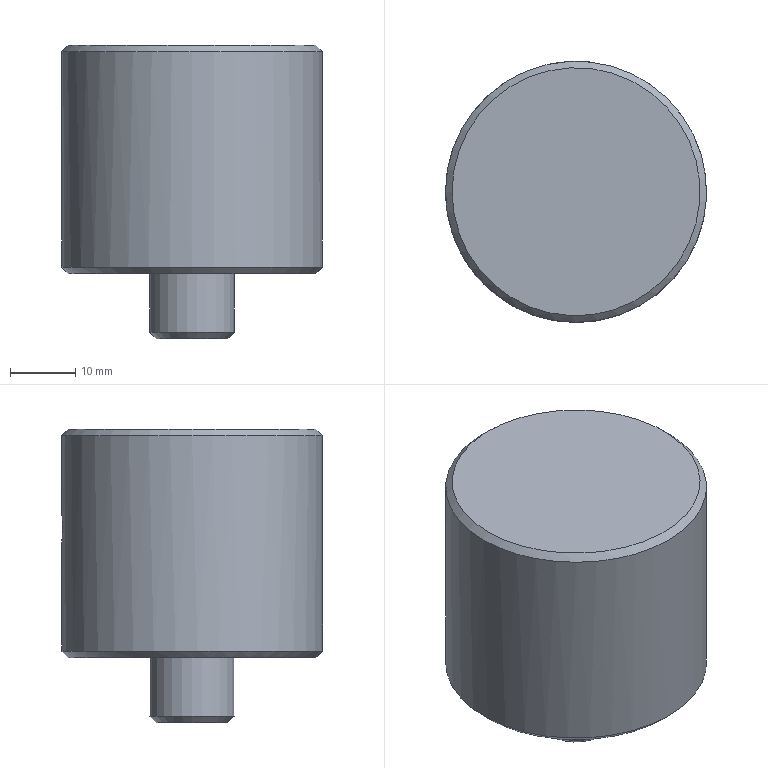Part | STEP file | gslz 2016.10.28-6_id186_x_t | 1 solid | 10 faces | box 40 x 40 x 45 mm | volume 44861 mm3 | cone 4 | cylinder 3 | plane 3 | commonest cylinder face diameters 5 x1 13 x1 40 x1
STEP:
#1=CARTESIAN_POINT('',(-310.,130.,30.992));
#2=VERTEX_POINT('',#1);
#3=CARTESIAN_POINT('',(-310.,150.,30.992));
#4=DIRECTION('',(0.,0.,-1.));
#5=DIRECTION('',(0.,-1.,0.));
#6=AXIS2_PLACEMENT_3D('',#3,#4,#5);
#7=CIRCLE('',#6,20.);
#8=EDGE_CURVE('',#2,#2,#7,.T.);
#9=ORIENTED_EDGE('',*,*,#8,.F.);
#10=EDGE_LOOP('',(#9));
#11=FACE_BOUND('',#10,.T.);
#12=CARTESIAN_POINT('',(-310.,130.,63.992));
#13=VERTEX_POINT('',#12);
#14=CARTESIAN_POINT('',(-310.,150.,63.992));
#15=DIRECTION('',(0.,0.,1.));
#16=DIRECTION('',(0.,-1.,0.));
#17=AXIS2_PLACEMENT_3D('',#14,#15,#16);
#18=CIRCLE('',#17,20.);
#19=EDGE_CURVE('',#13,#13,#18,.T.);
#20=ORIENTED_EDGE('',*,*,#19,.F.);
#21=EDGE_LOOP('',(#20));
#22=FACE_BOUND('',#21,.T.);
#23=CARTESIAN_POINT('',(-308.582,169.95,52.053));
#24=VERTEX_POINT('',#23);
#25=CARTESIAN_POINT('',(-308.582,169.95,52.053));
#26=CARTESIAN_POINT('',(-308.351,169.933,51.894));
#27=CARTESIAN_POINT('',(-308.145,169.914,51.693));
#28=CARTESIAN_POINT('',(-307.979,169.898,51.467));
#29=CARTESIAN_POINT('',(-307.814,169.881,51.241));
#30=CARTESIAN_POINT('',(-307.686,169.866,50.983));
#31=CARTESIAN_POINT('',(-307.605,169.856,50.714));
#32=CARTESIAN_POINT('',(-307.524,169.846,50.446));
#33=CARTESIAN_POINT('',(-307.488,169.842,50.161));
#34=CARTESIAN_POINT('',(-307.501,169.843,49.881));
#35=CARTESIAN_POINT('',(-307.513,169.845,49.604));
#36=CARTESIAN_POINT('',(-307.573,169.853,49.324));
#37=CARTESIAN_POINT('',(-307.676,169.865,49.066));
#38=CARTESIAN_POINT('',(-307.779,169.877,48.808));
#39=CARTESIAN_POINT('',(-307.928,169.893,48.564));
#40=CARTESIAN_POINT('',(-308.11,169.91,48.355));
#41=CARTESIAN_POINT('',(-308.293,169.928,48.143));
#42=CARTESIAN_POINT('',(-308.515,169.946,47.961));
#43=CARTESIAN_POINT('',(-308.758,169.961,47.822));
#44=CARTESIAN_POINT('',(-309.001,169.977,47.683));
#45=CARTESIAN_POINT('',(-309.272,169.989,47.584));
#46=CARTESIAN_POINT('',(-309.548,169.995,47.533));
#47=CARTESIAN_POINT('',(-309.823,170.001,47.483));
#48=CARTESIAN_POINT('',(-310.11,170.002,47.479));
#49=CARTESIAN_POINT('',(-310.385,169.996,47.523));
#50=CARTESIAN_POINT('',(-310.66,169.991,47.566));
#51=CARTESIAN_POINT('',(-310.93,169.98,47.656));
#52=CARTESIAN_POINT('',(-311.175,169.965,47.787));
#53=CARTESIAN_POINT('',(-311.421,169.951,47.918));
#54=CARTESIAN_POINT('',(-311.647,169.933,48.093));
#55=CARTESIAN_POINT('',(-311.836,169.916,48.297));
#56=CARTESIAN_POINT('',(-312.026,169.898,48.503));
#57=CARTESIAN_POINT('',(-312.183,169.881,48.744));
#58=CARTESIAN_POINT('',(-312.294,169.868,49.002));
#59=CARTESIAN_POINT('',(-312.405,169.855,49.259));
#60=CARTESIAN_POINT('',(-312.473,169.847,49.539));
#61=CARTESIAN_POINT('',(-312.492,169.844,49.819));
#62=CARTESIAN_POINT('',(-312.512,169.842,50.097));
#63=CARTESIAN_POINT('',(-312.484,169.845,50.382));
#64=CARTESIAN_POINT('',(-312.41,169.854,50.65));
#65=CARTESIAN_POINT('',(-312.337,169.863,50.918));
#66=CARTESIAN_POINT('',(-312.217,169.877,51.177));
#67=CARTESIAN_POINT('',(-312.061,169.894,51.406));
#68=CARTESIAN_POINT('',(-311.903,169.91,51.636));
#69=CARTESIAN_POINT('',(-311.704,169.929,51.842));
#70=CARTESIAN_POINT('',(-311.479,169.945,52.007));
#71=CARTESIAN_POINT('',(-311.253,169.962,52.173));
#72=CARTESIAN_POINT('',(-310.995,169.977,52.302));
#73=CARTESIAN_POINT('',(-310.727,169.987,52.384));
#74=CARTESIAN_POINT('',(-310.459,169.997,52.466));
#75=CARTESIAN_POINT('',(-310.174,170.001,52.502));
#76=CARTESIAN_POINT('',(-309.894,170.,52.49));
#77=CARTESIAN_POINT('',(-309.616,169.998,52.479));
#78=CARTESIAN_POINT('',(-309.337,169.991,52.419));
#79=CARTESIAN_POINT('',(-309.079,169.979,52.317));
#80=CARTESIAN_POINT('',(-308.904,169.971,52.248));
#81=CARTESIAN_POINT('',(-308.737,169.961,52.159));
#82=CARTESIAN_POINT('',(-308.582,169.95,52.053));
#83=B_SPLINE_CURVE_WITH_KNOTS('',3,(#25,#26,#27,#28,#29,#30,#31,#32,#33,#34,#35,#36,#37,#38,#39,#40,#41,#42,#43,#44,#45,#46,#47,#48,#49,#50,#51,#52,#53,#54,#55,#56,#57,#58,#59,#60,#61,#62,#63,#64,#65,#66,#67,#68,#69,#70,#71,#72,#73,#74,#75,#76,#77,#78,#79,#80,#81,#82),.UNSPECIFIED.,.T.,.F.,(1,3,3,3,3,3,3,3,3,3,3,3,3,3,3,3,3,3,3,3,3,1),(-0.03573,0.,0.05381,0.1076,0.1613,0.2146,0.2679,0.3216,0.3755,0.429,0.4822,0.5357,0.5895,0.6432,0.6966,0.7499,0.8035,0.8573,0.911,0.9643,1.,1.054),.UNSPECIFIED.);
#84=EDGE_CURVE('',#24,#24,#83,.T.);
#85=ORIENTED_EDGE('',*,*,#84,.F.);
#86=EDGE_LOOP('',(#85));
#87=FACE_BOUND('',#86,.T.);
#88=CARTESIAN_POINT('',(-310.,150.,69.992));
#89=DIRECTION('',(0.,0.,-1.));
#90=DIRECTION('',(-1.,0.,0.));
#91=AXIS2_PLACEMENT_3D('',#88,#89,#90);
#92=CYLINDRICAL_SURFACE('',#91,20.);
#93=ADVANCED_FACE('',(#11,#22,#87),#92,.T.);
#94=CARTESIAN_POINT('',(-303.5,150.,29.992));
#95=VERTEX_POINT('',#94);
#96=CARTESIAN_POINT('',(-310.,150.,29.992));
#97=DIRECTION('',(0.,0.,1.));
#98=DIRECTION('',(1.,0.,0.));
#99=AXIS2_PLACEMENT_3D('',#96,#97,#98);
#100=CIRCLE('',#99,6.5);
#101=EDGE_CURVE('',#95,#95,#100,.T.);
#102=ORIENTED_EDGE('',*,*,#101,.T.);
#103=EDGE_LOOP('',(#102));
#104=FACE_BOUND('',#103,.T.);
#105=CARTESIAN_POINT('',(-329.,150.,29.992));
#106=VERTEX_POINT('',#105);
#107=CARTESIAN_POINT('',(-310.,150.,29.992));
#108=DIRECTION('',(0.,0.,1.));
#109=DIRECTION('',(-1.,0.,0.));
#110=AXIS2_PLACEMENT_3D('',#107,#108,#109);
#111=CIRCLE('',#110,19.);
#112=EDGE_CURVE('',#106,#106,#111,.T.);
#113=ORIENTED_EDGE('',*,*,#112,.F.);
#114=EDGE_LOOP('',(#113));
#115=FACE_BOUND('',#114,.T.);
#116=CARTESIAN_POINT('',(-310.,150.,29.992));
#117=DIRECTION('',(0.,0.,1.));
#118=DIRECTION('',(0.,1.,0.));
#119=AXIS2_PLACEMENT_3D('',#116,#117,#118);
#120=PLANE('',#119);
#121=ADVANCED_FACE('',(#104,#115),#120,.F.);
#122=CARTESIAN_POINT('',(-329.,150.,64.992));
#123=VERTEX_POINT('',#122);
#124=CARTESIAN_POINT('',(-310.,150.,64.992));
#125=DIRECTION('',(0.,0.,-1.));
#126=DIRECTION('',(-1.,0.,0.));
#127=AXIS2_PLACEMENT_3D('',#124,#125,#126);
#128=CIRCLE('',#127,19.);
#129=EDGE_CURVE('',#123,#123,#128,.T.);
#130=ORIENTED_EDGE('',*,*,#129,.F.);
#131=EDGE_LOOP('',(#130));
#132=FACE_OUTER_BOUND('',#131,.T.);
#133=CARTESIAN_POINT('',(-310.,150.,64.992));
#134=DIRECTION('',(0.,0.,1.));
#135=DIRECTION('',(0.,1.,0.));
#136=AXIS2_PLACEMENT_3D('',#133,#134,#135);
#137=PLANE('',#136);
#138=ADVANCED_FACE('',(#132),#137,.T.);
#139=ORIENTED_EDGE('',*,*,#84,.T.);
#140=EDGE_LOOP('',(#139));
#141=FACE_BOUND('',#140,.T.);
#142=CARTESIAN_POINT('',(-307.499,154.9,49.992));
#143=VERTEX_POINT('',#142);
#144=CARTESIAN_POINT('',(-307.499,154.9,49.992));
#145=CARTESIAN_POINT('',(-307.499,154.9,50.272));
#146=CARTESIAN_POINT('',(-307.547,154.9,50.556));
#147=CARTESIAN_POINT('',(-307.64,154.9,50.82));
#148=CARTESIAN_POINT('',(-307.733,154.9,51.084));
#149=CARTESIAN_POINT('',(-307.872,154.9,51.336));
#150=CARTESIAN_POINT('',(-308.047,154.9,51.554));
#151=CARTESIAN_POINT('',(-308.222,154.9,51.773));
#152=CARTESIAN_POINT('',(-308.437,154.9,51.964));
#153=CARTESIAN_POINT('',(-308.674,154.9,52.112));
#154=CARTESIAN_POINT('',(-308.911,154.9,52.261));
#155=CARTESIAN_POINT('',(-309.177,154.9,52.37));
#156=CARTESIAN_POINT('',(-309.45,154.9,52.431));
#157=CARTESIAN_POINT('',(-309.723,154.9,52.493));
#158=CARTESIAN_POINT('',(-310.011,154.9,52.508));
#159=CARTESIAN_POINT('',(-310.289,154.9,52.476));
#160=CARTESIAN_POINT('',(-310.566,154.9,52.443));
#161=CARTESIAN_POINT('',(-310.843,154.9,52.362));
#162=CARTESIAN_POINT('',(-311.094,154.9,52.24));
#163=CARTESIAN_POINT('',(-311.346,154.9,52.117));
#164=CARTESIAN_POINT('',(-311.58,154.9,51.95));
#165=CARTESIAN_POINT('',(-311.776,154.9,51.751));
#166=CARTESIAN_POINT('',(-311.973,154.9,51.552));
#167=CARTESIAN_POINT('',(-312.138,154.9,51.316));
#168=CARTESIAN_POINT('',(-312.258,154.9,51.063));
#169=CARTESIAN_POINT('',(-312.378,154.9,50.81));
#170=CARTESIAN_POINT('',(-312.456,154.9,50.533));
#171=CARTESIAN_POINT('',(-312.485,154.9,50.255));
#172=CARTESIAN_POINT('',(-312.515,154.9,49.977));
#173=CARTESIAN_POINT('',(-312.496,154.9,49.69));
#174=CARTESIAN_POINT('',(-312.432,154.9,49.417));
#175=CARTESIAN_POINT('',(-312.368,154.9,49.145));
#176=CARTESIAN_POINT('',(-312.255,154.9,48.88));
#177=CARTESIAN_POINT('',(-312.105,154.9,48.645));
#178=CARTESIAN_POINT('',(-311.954,154.9,48.409));
#179=CARTESIAN_POINT('',(-311.76,154.9,48.196));
#180=CARTESIAN_POINT('',(-311.54,154.9,48.024));
#181=CARTESIAN_POINT('',(-311.319,154.9,47.851));
#182=CARTESIAN_POINT('',(-311.066,154.9,47.714));
#183=CARTESIAN_POINT('',(-310.801,154.9,47.625));
#184=CARTESIAN_POINT('',(-310.536,154.9,47.535));
#185=CARTESIAN_POINT('',(-310.252,154.9,47.49));
#186=CARTESIAN_POINT('',(-309.972,154.9,47.493));
#187=CARTESIAN_POINT('',(-309.692,154.9,47.496));
#188=CARTESIAN_POINT('',(-309.409,154.9,47.547));
#189=CARTESIAN_POINT('',(-309.146,154.9,47.642));
#190=CARTESIAN_POINT('',(-308.883,154.9,47.738));
#191=CARTESIAN_POINT('',(-308.633,154.9,47.88));
#192=CARTESIAN_POINT('',(-308.416,154.9,48.057));
#193=CARTESIAN_POINT('',(-308.2,154.9,48.234));
#194=CARTESIAN_POINT('',(-308.011,154.9,48.451));
#195=CARTESIAN_POINT('',(-307.865,154.9,48.69));
#196=CARTESIAN_POINT('',(-307.719,154.9,48.929));
#197=CARTESIAN_POINT('',(-307.613,154.9,49.196));
#198=CARTESIAN_POINT('',(-307.554,154.9,49.47));
#199=CARTESIAN_POINT('',(-307.518,154.9,49.641));
#200=CARTESIAN_POINT('',(-307.499,154.9,49.817));
#201=CARTESIAN_POINT('',(-307.499,154.9,49.992));
#202=B_SPLINE_CURVE_WITH_KNOTS('',3,(#144,#145,#146,#147,#148,#149,#150,#151,#152,#153,#154,#155,#156,#157,#158,#159,#160,#161,#162,#163,#164,#165,#166,#167,#168,#169,#170,#171,#172,#173,#174,#175,#176,#177,#178,#179,#180,#181,#182,#183,#184,#185,#186,#187,#188,#189,#190,#191,#192,#193,#194,#195,#196,#197,#198,#199,#200,#201),.UNSPECIFIED.,.T.,.F.,(1,3,3,3,3,3,3,3,3,3,3,3,3,3,3,3,3,3,3,3,3,1),(-0.03332,0.,0.0537,0.1074,0.1611,0.2148,0.2685,0.3222,0.3759,0.4296,0.4833,0.537,0.5907,0.6445,0.6982,0.7519,0.8056,0.8593,0.913,0.9667,1.,1.054),.UNSPECIFIED.);
#203=EDGE_CURVE('',#143,#143,#202,.T.);
#204=ORIENTED_EDGE('',*,*,#203,.T.);
#205=EDGE_LOOP('',(#204));
#206=FACE_BOUND('',#205,.T.);
#207=CARTESIAN_POINT('',(-309.997,200.,49.992));
#208=DIRECTION('',(-0.00004493,-1.,0.));
#209=DIRECTION('',(1.,-0.00004493,0.));
#210=AXIS2_PLACEMENT_3D('',#207,#208,#209);
#211=CYLINDRICAL_SURFACE('',#210,2.5);
#212=ADVANCED_FACE('',(#141,#206),#211,.F.);
#213=ORIENTED_EDGE('',*,*,#203,.F.);
#214=EDGE_LOOP('',(#213));
#215=FACE_BOUND('',#214,.T.);
#216=CARTESIAN_POINT('',(-309.999,153.398,49.992));
#217=VERTEX_POINT('',#216);
#218=VERTEX_LOOP('',#217);
#219=FACE_BOUND('',#218,.T.);
#220=CARTESIAN_POINT('',(-309.999,154.9,49.992));
#221=DIRECTION('',(0.00004493,1.,0.));
#222=DIRECTION('',(-1.,0.00004493,0.));
#223=AXIS2_PLACEMENT_3D('',#220,#221,#222);
#224=CONICAL_SURFACE('',#223,2.5,59.);
#225=ADVANCED_FACE('',(#215,#219),#224,.F.);
#226=ORIENTED_EDGE('',*,*,#8,.T.);
#227=EDGE_LOOP('',(#226));
#228=FACE_BOUND('',#227,.T.);
#229=ORIENTED_EDGE('',*,*,#112,.T.);
#230=EDGE_LOOP('',(#229));
#231=FACE_BOUND('',#230,.T.);
#232=CARTESIAN_POINT('',(-310.,150.,29.992));
#233=DIRECTION('',(0.,0.,1.));
#234=DIRECTION('',(0.,-1.,0.));
#235=AXIS2_PLACEMENT_3D('',#232,#233,#234);
#236=CONICAL_SURFACE('',#235,19.,45.);
#237=ADVANCED_FACE('',(#228,#231),#236,.T.);
#238=ORIENTED_EDGE('',*,*,#129,.T.);
#239=EDGE_LOOP('',(#238));
#240=FACE_BOUND('',#239,.T.);
#241=ORIENTED_EDGE('',*,*,#19,.T.);
#242=EDGE_LOOP('',(#241));
#243=FACE_BOUND('',#242,.T.);
#244=CARTESIAN_POINT('',(-310.,150.,63.992));
#245=DIRECTION('',(0.,0.,-1.));
#246=DIRECTION('',(0.,1.,0.));
#247=AXIS2_PLACEMENT_3D('',#244,#245,#246);
#248=CONICAL_SURFACE('',#247,20.,45.);
#249=ADVANCED_FACE('',(#240,#243),#248,.T.);
#250=CARTESIAN_POINT('',(-304.5,150.,19.992));
#251=VERTEX_POINT('',#250);
#252=CARTESIAN_POINT('',(-310.,150.,19.992));
#253=DIRECTION('',(0.,0.,1.));
#254=DIRECTION('',(1.,0.,0.));
#255=AXIS2_PLACEMENT_3D('',#252,#253,#254);
#256=CIRCLE('',#255,5.5);
#257=EDGE_CURVE('',#251,#251,#256,.T.);
#258=ORIENTED_EDGE('',*,*,#257,.F.);
#259=EDGE_LOOP('',(#258));
#260=FACE_OUTER_BOUND('',#259,.T.);
#261=CARTESIAN_POINT('',(-310.,150.,19.992));
#262=DIRECTION('',(0.,0.,-1.));
#263=DIRECTION('',(-1.,0.,0.));
#264=AXIS2_PLACEMENT_3D('',#261,#262,#263);
#265=PLANE('',#264);
#266=ADVANCED_FACE('',(#260),#265,.T.);
#267=CARTESIAN_POINT('',(-303.5,150.,20.992));
#268=VERTEX_POINT('',#267);
#269=CARTESIAN_POINT('',(-310.,150.,20.992));
#270=DIRECTION('',(0.,0.,-1.));
#271=DIRECTION('',(1.,0.,0.));
#272=AXIS2_PLACEMENT_3D('',#269,#270,#271);
#273=CIRCLE('',#272,6.5);
#274=EDGE_CURVE('',#268,#268,#273,.T.);
#275=ORIENTED_EDGE('',*,*,#274,.F.);
#276=EDGE_LOOP('',(#275));
#277=FACE_BOUND('',#276,.T.);
#278=ORIENTED_EDGE('',*,*,#101,.F.);
#279=EDGE_LOOP('',(#278));
#280=FACE_BOUND('',#279,.T.);
#281=CARTESIAN_POINT('',(-310.,150.,29.992));
#282=DIRECTION('',(0.,0.,-1.));
#283=DIRECTION('',(-1.,0.,0.));
#284=AXIS2_PLACEMENT_3D('',#281,#282,#283);
#285=CYLINDRICAL_SURFACE('',#284,6.5);
#286=ADVANCED_FACE('',(#277,#280),#285,.T.);
#287=ORIENTED_EDGE('',*,*,#257,.T.);
#288=EDGE_LOOP('',(#287));
#289=FACE_BOUND('',#288,.T.);
#290=ORIENTED_EDGE('',*,*,#274,.T.);
#291=EDGE_LOOP('',(#290));
#292=FACE_BOUND('',#291,.T.);
#293=CARTESIAN_POINT('',(-310.,150.,20.992));
#294=DIRECTION('',(0.,0.,1.));
#295=DIRECTION('',(-1.,0.,0.));
#296=AXIS2_PLACEMENT_3D('',#293,#294,#295);
#297=CONICAL_SURFACE('',#296,6.5,45.);
#298=ADVANCED_FACE('',(#289,#292),#297,.T.);
#299=CLOSED_SHELL('',(#93,#121,#138,#212,#225,#237,#249,#266,#286,#298));
#300=MANIFOLD_SOLID_BREP('',#299);
#301=(LENGTH_UNIT()NAMED_UNIT(*)SI_UNIT(.MILLI.,.METRE.));
#302=UNCERTAINTY_MEASURE_WITH_UNIT(LENGTH_MEASURE(0.0508),#301,'','');
#303=(NAMED_UNIT(*)PLANE_ANGLE_UNIT()SI_UNIT($,.RADIAN.));
#304=PLANE_ANGLE_MEASURE_WITH_UNIT(PLANE_ANGLE_MEASURE(0.01745),#303);
#305=DIMENSIONAL_EXPONENTS(0.,0.,0.,0.,0.,0.,0.);
#306=(CONVERSION_BASED_UNIT('DEGREE',#304)NAMED_UNIT(#305)PLANE_ANGLE_UNIT());
#307=(NAMED_UNIT(*)SI_UNIT($,.STERADIAN.)SOLID_ANGLE_UNIT());
#308=(GEOMETRIC_REPRESENTATION_CONTEXT(3)GLOBAL_UNCERTAINTY_ASSIGNED_CONTEXT((#302))GLOBAL_UNIT_ASSIGNED_CONTEXT((#301,#306,#307))REPRESENTATION_CONTEXT('',''));
#309=ADVANCED_BREP_SHAPE_REPRESENTATION('',(#300),#308);